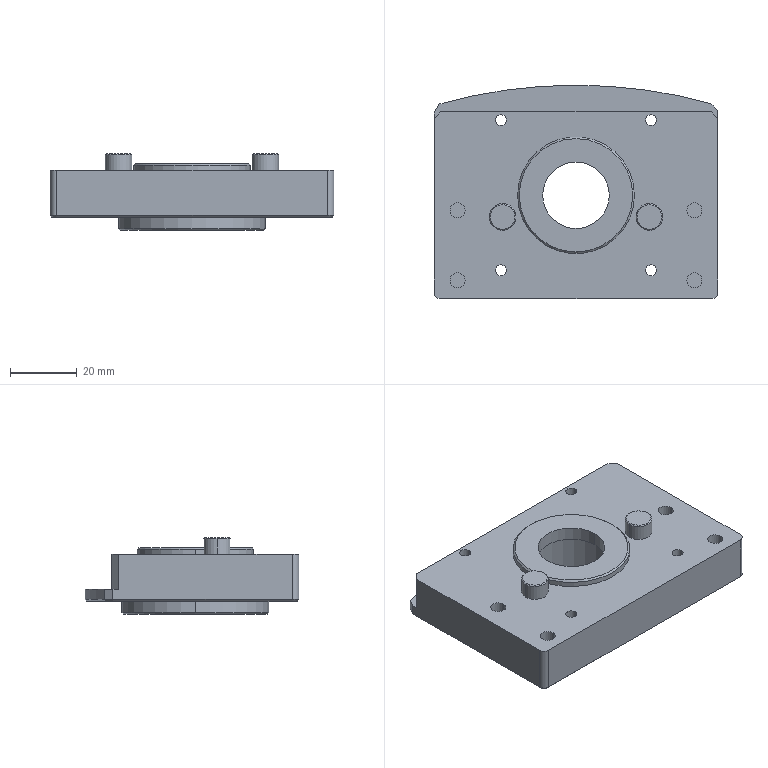Part | SolidWorks | features BaseBody 1 | 1 solid | 99 faces | box 85 x 64 x 23 mm | volume 64137 mm3 | cylinder 51 | plane 33 | cone 15 | commonest cylinder face diameters 3.3 x12 8 x12 4.5 x8 7 x8 4 x2 20 x2